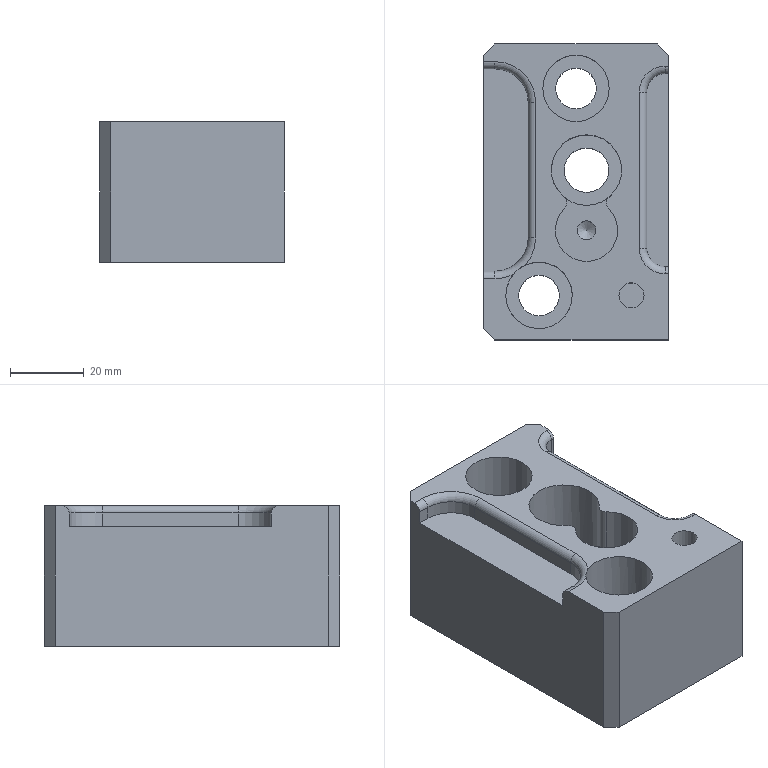Part | STEP file | 1_id102_x_t | 1 solid | 48 faces | box 50 x 80 x 38.1 mm | volume 121881 mm3 | plane 22 | cylinder 21 | torus 4 | cone 1 | commonest cylinder face diameters 4 x8 18 x4 10 x2 11 x2 5.105 x1 6.8 x1